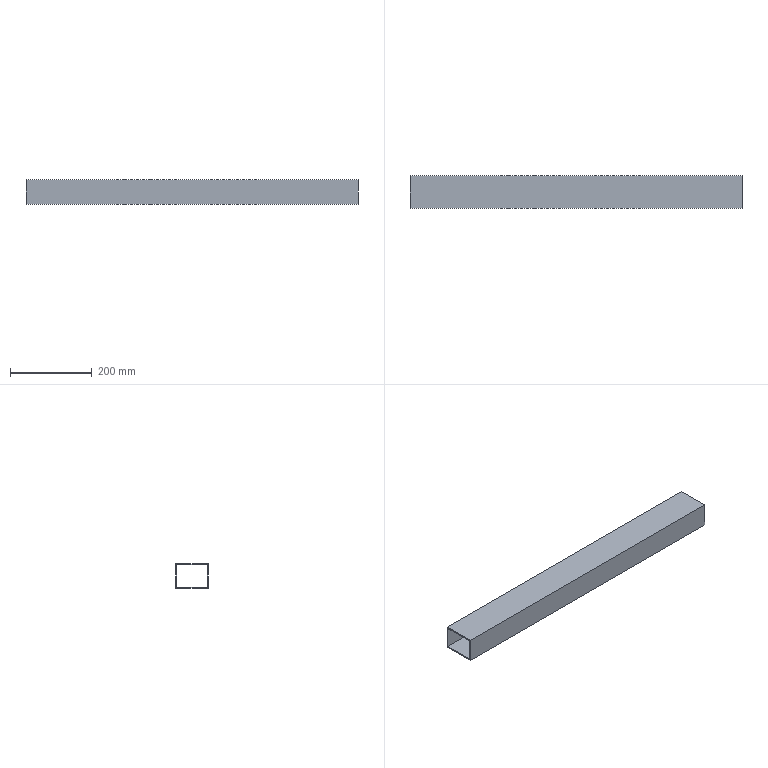Part | STEP file | Guide wheel mechanism revised.sldasm-Part-7 | 1 solid | 10 faces | box 810 x 80 x 60 mm | volume 651240 mm3 | plane 10
STEP:
#1=CARTESIAN_POINT('',(405.,820.,-505.));
#2=VERTEX_POINT('',#1);
#3=CARTESIAN_POINT('',(405.,820.,-445.));
#4=VERTEX_POINT('',#3);
#5=CARTESIAN_POINT('',(405.,820.,-445.));
#6=DIRECTION('',(0.,0.,1.));
#7=VECTOR('',#6,1000.);
#8=LINE('',#5,#7);
#9=EDGE_CURVE('',#2,#4,#8,.T.);
#10=ORIENTED_EDGE('',*,*,#9,.F.);
#11=CARTESIAN_POINT('',(-405.,820.,-505.));
#12=VERTEX_POINT('',#11);
#13=CARTESIAN_POINT('',(505.,820.,-505.));
#14=DIRECTION('',(-1.,0.,0.));
#15=VECTOR('',#14,1000.);
#16=LINE('',#13,#15);
#17=EDGE_CURVE('',#2,#12,#16,.T.);
#18=ORIENTED_EDGE('',*,*,#17,.T.);
#19=CARTESIAN_POINT('',(-405.,820.,-445.));
#20=VERTEX_POINT('',#19);
#21=CARTESIAN_POINT('',(-405.,820.,-445.));
#22=DIRECTION('',(0.,0.,1.));
#23=VECTOR('',#22,1000.);
#24=LINE('',#21,#23);
#25=EDGE_CURVE('',#12,#20,#24,.T.);
#26=ORIENTED_EDGE('',*,*,#25,.T.);
#27=CARTESIAN_POINT('',(505.,820.,-445.));
#28=DIRECTION('',(-1.,0.,0.));
#29=VECTOR('',#28,1000.);
#30=LINE('',#27,#29);
#31=EDGE_CURVE('',#4,#20,#30,.T.);
#32=ORIENTED_EDGE('',*,*,#31,.F.);
#33=EDGE_LOOP('',(#10,#18,#26,#32));
#34=FACE_OUTER_BOUND('',#33,.T.);
#35=CARTESIAN_POINT('',(505.,820.,-445.));
#36=DIRECTION('',(0.,-1.,0.));
#37=DIRECTION('',(0.,0.,-1.));
#38=AXIS2_PLACEMENT_3D('',#35,#36,#37);
#39=PLANE('',#38);
#40=ADVANCED_FACE('',(#34),#39,.F.);
#41=CARTESIAN_POINT('',(405.,740.,-505.));
#42=VERTEX_POINT('',#41);
#43=CARTESIAN_POINT('',(405.,820.,-505.));
#44=DIRECTION('',(0.,1.,0.));
#45=VECTOR('',#44,1000.);
#46=LINE('',#43,#45);
#47=EDGE_CURVE('',#42,#2,#46,.T.);
#48=ORIENTED_EDGE('',*,*,#47,.F.);
#49=CARTESIAN_POINT('',(-405.,740.,-505.));
#50=VERTEX_POINT('',#49);
#51=CARTESIAN_POINT('',(505.,740.,-505.));
#52=DIRECTION('',(-1.,0.,0.));
#53=VECTOR('',#52,1000.);
#54=LINE('',#51,#53);
#55=EDGE_CURVE('',#42,#50,#54,.T.);
#56=ORIENTED_EDGE('',*,*,#55,.T.);
#57=CARTESIAN_POINT('',(-405.,820.,-505.));
#58=DIRECTION('',(0.,1.,0.));
#59=VECTOR('',#58,1000.);
#60=LINE('',#57,#59);
#61=EDGE_CURVE('',#50,#12,#60,.T.);
#62=ORIENTED_EDGE('',*,*,#61,.T.);
#63=ORIENTED_EDGE('',*,*,#17,.F.);
#64=EDGE_LOOP('',(#48,#56,#62,#63));
#65=FACE_OUTER_BOUND('',#64,.T.);
#66=CARTESIAN_POINT('',(505.,820.,-505.));
#67=DIRECTION('',(0.,0.,1.));
#68=DIRECTION('',(1.,0.,0.));
#69=AXIS2_PLACEMENT_3D('',#66,#67,#68);
#70=PLANE('',#69);
#71=ADVANCED_FACE('',(#65),#70,.F.);
#72=CARTESIAN_POINT('',(405.,740.,-445.));
#73=VERTEX_POINT('',#72);
#74=CARTESIAN_POINT('',(405.,740.,-445.));
#75=DIRECTION('',(0.,0.,-1.));
#76=VECTOR('',#75,1000.);
#77=LINE('',#74,#76);
#78=EDGE_CURVE('',#73,#42,#77,.T.);
#79=ORIENTED_EDGE('',*,*,#78,.F.);
#80=CARTESIAN_POINT('',(-405.,740.,-445.));
#81=VERTEX_POINT('',#80);
#82=CARTESIAN_POINT('',(505.,740.,-445.));
#83=DIRECTION('',(-1.,0.,0.));
#84=VECTOR('',#83,1000.);
#85=LINE('',#82,#84);
#86=EDGE_CURVE('',#73,#81,#85,.T.);
#87=ORIENTED_EDGE('',*,*,#86,.T.);
#88=CARTESIAN_POINT('',(-405.,740.,-445.));
#89=DIRECTION('',(0.,0.,-1.));
#90=VECTOR('',#89,1000.);
#91=LINE('',#88,#90);
#92=EDGE_CURVE('',#81,#50,#91,.T.);
#93=ORIENTED_EDGE('',*,*,#92,.T.);
#94=ORIENTED_EDGE('',*,*,#55,.F.);
#95=EDGE_LOOP('',(#79,#87,#93,#94));
#96=FACE_OUTER_BOUND('',#95,.T.);
#97=CARTESIAN_POINT('',(505.,740.,-445.));
#98=DIRECTION('',(0.,1.,0.));
#99=DIRECTION('',(0.,0.,1.));
#100=AXIS2_PLACEMENT_3D('',#97,#98,#99);
#101=PLANE('',#100);
#102=ADVANCED_FACE('',(#96),#101,.F.);
#103=CARTESIAN_POINT('',(405.,820.,-445.));
#104=DIRECTION('',(0.,-1.,0.));
#105=VECTOR('',#104,1000.);
#106=LINE('',#103,#105);
#107=EDGE_CURVE('',#4,#73,#106,.T.);
#108=ORIENTED_EDGE('',*,*,#107,.F.);
#109=ORIENTED_EDGE('',*,*,#31,.T.);
#110=CARTESIAN_POINT('',(-405.,820.,-445.));
#111=DIRECTION('',(0.,-1.,0.));
#112=VECTOR('',#111,1000.);
#113=LINE('',#110,#112);
#114=EDGE_CURVE('',#20,#81,#113,.T.);
#115=ORIENTED_EDGE('',*,*,#114,.T.);
#116=ORIENTED_EDGE('',*,*,#86,.F.);
#117=EDGE_LOOP('',(#108,#109,#115,#116));
#118=FACE_OUTER_BOUND('',#117,.T.);
#119=CARTESIAN_POINT('',(505.,820.,-445.));
#120=DIRECTION('',(0.,0.,-1.));
#121=DIRECTION('',(0.,1.,0.));
#122=AXIS2_PLACEMENT_3D('',#119,#120,#121);
#123=PLANE('',#122);
#124=ADVANCED_FACE('',(#118),#123,.F.);
#125=ORIENTED_EDGE('',*,*,#114,.F.);
#126=ORIENTED_EDGE('',*,*,#25,.F.);
#127=ORIENTED_EDGE('',*,*,#61,.F.);
#128=ORIENTED_EDGE('',*,*,#92,.F.);
#129=EDGE_LOOP('',(#125,#126,#127,#128));
#130=FACE_OUTER_BOUND('',#129,.T.);
#131=CARTESIAN_POINT('',(-405.,817.,-448.));
#132=VERTEX_POINT('',#131);
#133=CARTESIAN_POINT('',(-405.,743.,-448.));
#134=VERTEX_POINT('',#133);
#135=CARTESIAN_POINT('',(-405.,817.,-448.));
#136=DIRECTION('',(0.,-1.,0.));
#137=VECTOR('',#136,1000.);
#138=LINE('',#135,#137);
#139=EDGE_CURVE('',#132,#134,#138,.T.);
#140=ORIENTED_EDGE('',*,*,#139,.T.);
#141=CARTESIAN_POINT('',(-405.,743.,-502.));
#142=VERTEX_POINT('',#141);
#143=CARTESIAN_POINT('',(-405.,743.,-448.));
#144=DIRECTION('',(0.,0.,-1.));
#145=VECTOR('',#144,1000.);
#146=LINE('',#143,#145);
#147=EDGE_CURVE('',#134,#142,#146,.T.);
#148=ORIENTED_EDGE('',*,*,#147,.T.);
#149=CARTESIAN_POINT('',(-405.,817.,-502.));
#150=VERTEX_POINT('',#149);
#151=CARTESIAN_POINT('',(-405.,817.,-502.));
#152=DIRECTION('',(0.,1.,0.));
#153=VECTOR('',#152,1000.);
#154=LINE('',#151,#153);
#155=EDGE_CURVE('',#142,#150,#154,.T.);
#156=ORIENTED_EDGE('',*,*,#155,.T.);
#157=CARTESIAN_POINT('',(-405.,817.,-448.));
#158=DIRECTION('',(0.,0.,1.));
#159=VECTOR('',#158,1000.);
#160=LINE('',#157,#159);
#161=EDGE_CURVE('',#150,#132,#160,.T.);
#162=ORIENTED_EDGE('',*,*,#161,.T.);
#163=EDGE_LOOP('',(#140,#148,#156,#162));
#164=FACE_BOUND('',#163,.T.);
#165=CARTESIAN_POINT('',(-405.,0.,0.));
#166=DIRECTION('',(1.,0.,0.));
#167=DIRECTION('',(0.,0.,-1.));
#168=AXIS2_PLACEMENT_3D('',#165,#166,#167);
#169=PLANE('',#168);
#170=ADVANCED_FACE('',(#130,#164),#169,.F.);
#171=CARTESIAN_POINT('',(405.,817.,-502.));
#172=VERTEX_POINT('',#171);
#173=CARTESIAN_POINT('',(505.,817.,-502.));
#174=DIRECTION('',(-1.,0.,0.));
#175=VECTOR('',#174,1000.);
#176=LINE('',#173,#175);
#177=EDGE_CURVE('',#172,#150,#176,.T.);
#178=ORIENTED_EDGE('',*,*,#177,.F.);
#179=CARTESIAN_POINT('',(405.,817.,-448.));
#180=VERTEX_POINT('',#179);
#181=CARTESIAN_POINT('',(405.,817.,-448.));
#182=DIRECTION('',(0.,0.,1.));
#183=VECTOR('',#182,1000.);
#184=LINE('',#181,#183);
#185=EDGE_CURVE('',#172,#180,#184,.T.);
#186=ORIENTED_EDGE('',*,*,#185,.T.);
#187=CARTESIAN_POINT('',(505.,817.,-448.));
#188=DIRECTION('',(-1.,0.,0.));
#189=VECTOR('',#188,1000.);
#190=LINE('',#187,#189);
#191=EDGE_CURVE('',#180,#132,#190,.T.);
#192=ORIENTED_EDGE('',*,*,#191,.T.);
#193=ORIENTED_EDGE('',*,*,#161,.F.);
#194=EDGE_LOOP('',(#178,#186,#192,#193));
#195=FACE_OUTER_BOUND('',#194,.T.);
#196=CARTESIAN_POINT('',(505.,817.,-448.));
#197=DIRECTION('',(0.,-1.,0.));
#198=DIRECTION('',(0.,0.,-1.));
#199=AXIS2_PLACEMENT_3D('',#196,#197,#198);
#200=PLANE('',#199);
#201=ADVANCED_FACE('',(#195),#200,.T.);
#202=CARTESIAN_POINT('',(405.,743.,-502.));
#203=VERTEX_POINT('',#202);
#204=CARTESIAN_POINT('',(505.,743.,-502.));
#205=DIRECTION('',(-1.,0.,0.));
#206=VECTOR('',#205,1000.);
#207=LINE('',#204,#206);
#208=EDGE_CURVE('',#203,#142,#207,.T.);
#209=ORIENTED_EDGE('',*,*,#208,.F.);
#210=CARTESIAN_POINT('',(405.,817.,-502.));
#211=DIRECTION('',(0.,1.,0.));
#212=VECTOR('',#211,1000.);
#213=LINE('',#210,#212);
#214=EDGE_CURVE('',#203,#172,#213,.T.);
#215=ORIENTED_EDGE('',*,*,#214,.T.);
#216=ORIENTED_EDGE('',*,*,#177,.T.);
#217=ORIENTED_EDGE('',*,*,#155,.F.);
#218=EDGE_LOOP('',(#209,#215,#216,#217));
#219=FACE_OUTER_BOUND('',#218,.T.);
#220=CARTESIAN_POINT('',(505.,817.,-502.));
#221=DIRECTION('',(0.,0.,1.));
#222=DIRECTION('',(1.,0.,0.));
#223=AXIS2_PLACEMENT_3D('',#220,#221,#222);
#224=PLANE('',#223);
#225=ADVANCED_FACE('',(#219),#224,.T.);
#226=CARTESIAN_POINT('',(405.,743.,-448.));
#227=VERTEX_POINT('',#226);
#228=CARTESIAN_POINT('',(505.,743.,-448.));
#229=DIRECTION('',(-1.,0.,0.));
#230=VECTOR('',#229,1000.);
#231=LINE('',#228,#230);
#232=EDGE_CURVE('',#227,#134,#231,.T.);
#233=ORIENTED_EDGE('',*,*,#232,.F.);
#234=CARTESIAN_POINT('',(405.,743.,-448.));
#235=DIRECTION('',(0.,0.,-1.));
#236=VECTOR('',#235,1000.);
#237=LINE('',#234,#236);
#238=EDGE_CURVE('',#227,#203,#237,.T.);
#239=ORIENTED_EDGE('',*,*,#238,.T.);
#240=ORIENTED_EDGE('',*,*,#208,.T.);
#241=ORIENTED_EDGE('',*,*,#147,.F.);
#242=EDGE_LOOP('',(#233,#239,#240,#241));
#243=FACE_OUTER_BOUND('',#242,.T.);
#244=CARTESIAN_POINT('',(505.,743.,-448.));
#245=DIRECTION('',(0.,1.,0.));
#246=DIRECTION('',(0.,0.,1.));
#247=AXIS2_PLACEMENT_3D('',#244,#245,#246);
#248=PLANE('',#247);
#249=ADVANCED_FACE('',(#243),#248,.T.);
#250=ORIENTED_EDGE('',*,*,#191,.F.);
#251=CARTESIAN_POINT('',(405.,817.,-448.));
#252=DIRECTION('',(0.,-1.,0.));
#253=VECTOR('',#252,1000.);
#254=LINE('',#251,#253);
#255=EDGE_CURVE('',#180,#227,#254,.T.);
#256=ORIENTED_EDGE('',*,*,#255,.T.);
#257=ORIENTED_EDGE('',*,*,#232,.T.);
#258=ORIENTED_EDGE('',*,*,#139,.F.);
#259=EDGE_LOOP('',(#250,#256,#257,#258));
#260=FACE_OUTER_BOUND('',#259,.T.);
#261=CARTESIAN_POINT('',(505.,817.,-448.));
#262=DIRECTION('',(0.,0.,-1.));
#263=DIRECTION('',(0.,1.,0.));
#264=AXIS2_PLACEMENT_3D('',#261,#262,#263);
#265=PLANE('',#264);
#266=ADVANCED_FACE('',(#260),#265,.T.);
#267=ORIENTED_EDGE('',*,*,#255,.F.);
#268=ORIENTED_EDGE('',*,*,#185,.F.);
#269=ORIENTED_EDGE('',*,*,#214,.F.);
#270=ORIENTED_EDGE('',*,*,#238,.F.);
#271=EDGE_LOOP('',(#267,#268,#269,#270));
#272=FACE_BOUND('',#271,.T.);
#273=ORIENTED_EDGE('',*,*,#9,.T.);
#274=ORIENTED_EDGE('',*,*,#107,.T.);
#275=ORIENTED_EDGE('',*,*,#78,.T.);
#276=ORIENTED_EDGE('',*,*,#47,.T.);
#277=EDGE_LOOP('',(#273,#274,#275,#276));
#278=FACE_OUTER_BOUND('',#277,.T.);
#279=CARTESIAN_POINT('',(405.,1970.,505.));
#280=DIRECTION('',(1.,0.,0.));
#281=DIRECTION('',(0.,0.,-1.));
#282=AXIS2_PLACEMENT_3D('',#279,#280,#281);
#283=PLANE('',#282);
#284=ADVANCED_FACE('',(#272,#278),#283,.T.);
#285=CLOSED_SHELL('',(#40,#71,#102,#124,#170,#201,#225,#249,#266,#284));
#286=MANIFOLD_SOLID_BREP('',#285);
#287=CARTESIAN_POINT('',(0.,0.,0.));
#288=DIRECTION('',(0.,0.,1.));
#289=DIRECTION('',(1.,0.,0.));
#290=AXIS2_PLACEMENT_3D('',#287,#288,#289);
#291=(LENGTH_UNIT()NAMED_UNIT(*)SI_UNIT(.MILLI.,.METRE.));
#292=UNCERTAINTY_MEASURE_WITH_UNIT(LENGTH_MEASURE(0.00001),#291,'','');
#293=(NAMED_UNIT(*)PLANE_ANGLE_UNIT()SI_UNIT($,.RADIAN.));
#294=(NAMED_UNIT(*)SI_UNIT($,.STERADIAN.)SOLID_ANGLE_UNIT());
#295=(GEOMETRIC_REPRESENTATION_CONTEXT(3)GLOBAL_UNCERTAINTY_ASSIGNED_CONTEXT((#292))GLOBAL_UNIT_ASSIGNED_CONTEXT((#291,#293,#294))REPRESENTATION_CONTEXT('',''));
#296=ADVANCED_BREP_SHAPE_REPRESENTATION('',(#286,#290),#295);